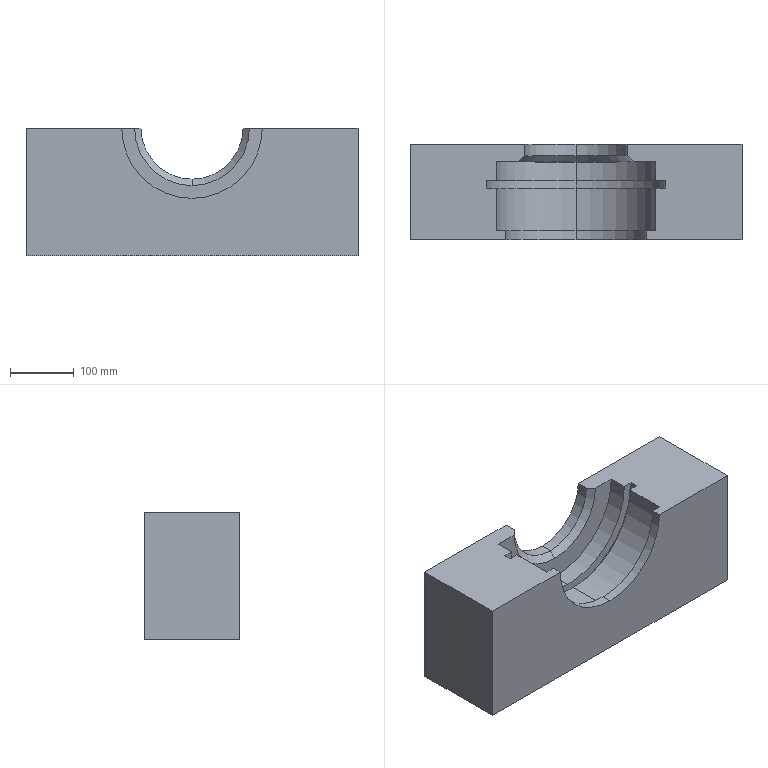Part | SolidWorks | features Chamfer 1, Extrusion 1, HoleWzd 1, RevCut 1 | 1 solid | 41 faces | box 520 x 150 x 200 mm | volume 12315251 mm3 | cylinder 16 | cone 14 | plane 11 | commonest cylinder face diameters 10.2 x6 250 x4 160 x2 220 x2 280 x2
STEP:
#1=CARTESIAN_POINT('',(-260.,132.,-80.));
#2=VERTEX_POINT('',#1);
#3=CARTESIAN_POINT('',(-180.,132.,0.));
#4=VERTEX_POINT('',#3);
#5=CARTESIAN_POINT('',(-260.,132.,0.));
#6=DIRECTION('',(0.,-1.,0.));
#7=DIRECTION('',(0.,0.,-1.));
#8=AXIS2_PLACEMENT_3D('',#5,#6,#7);
#9=CIRCLE('',#8,80.);
#10=EDGE_CURVE('',#2,#4,#9,.T.);
#11=ORIENTED_EDGE('',*,*,#10,.F.);
#12=CARTESIAN_POINT('',(-260.,122.,-90.));
#13=VERTEX_POINT('',#12);
#14=CARTESIAN_POINT('',(-260.,132.,-80.));
#15=DIRECTION('',(0.,-0.7071,-0.7071));
#16=VECTOR('',#15,1000.);
#17=LINE('',#14,#16);
#18=EDGE_CURVE('',#2,#13,#17,.T.);
#19=ORIENTED_EDGE('',*,*,#18,.T.);
#20=CARTESIAN_POINT('',(-170.,122.,0.));
#21=VERTEX_POINT('',#20);
#22=CARTESIAN_POINT('',(-260.,122.,0.));
#23=DIRECTION('',(0.,1.,0.));
#24=DIRECTION('',(0.,0.,-1.));
#25=AXIS2_PLACEMENT_3D('',#22,#23,#24);
#26=CIRCLE('',#25,90.);
#27=EDGE_CURVE('',#21,#13,#26,.T.);
#28=ORIENTED_EDGE('',*,*,#27,.F.);
#29=CARTESIAN_POINT('',(-260.,212.,0.));
#30=DIRECTION('',(0.7071,-0.7071,0.));
#31=VECTOR('',#30,1000.);
#32=LINE('',#29,#31);
#33=EDGE_CURVE('',#4,#21,#32,.T.);
#34=ORIENTED_EDGE('',*,*,#33,.F.);
#35=EDGE_LOOP('',(#11,#19,#28,#34));
#36=FACE_OUTER_BOUND('',#35,.T.);
#37=CARTESIAN_POINT('',(-260.,132.,0.));
#38=DIRECTION('',(0.,-1.,0.));
#39=DIRECTION('',(0.,0.,-1.));
#40=AXIS2_PLACEMENT_3D('',#37,#38,#39);
#41=CONICAL_SURFACE('',#40,80.,0.7854);
#42=ADVANCED_FACE('',(#36),#41,.F.);
#43=CARTESIAN_POINT('',(-260.,15.,-110.));
#44=VERTEX_POINT('',#43);
#45=CARTESIAN_POINT('',(-150.,15.,0.));
#46=VERTEX_POINT('',#45);
#47=CARTESIAN_POINT('',(-260.,15.,0.));
#48=DIRECTION('',(0.,-1.,0.));
#49=DIRECTION('',(0.,0.,-1.));
#50=AXIS2_PLACEMENT_3D('',#47,#48,#49);
#51=CIRCLE('',#50,110.);
#52=EDGE_CURVE('',#44,#46,#51,.T.);
#53=ORIENTED_EDGE('',*,*,#52,.F.);
#54=CARTESIAN_POINT('',(-260.,0.,-110.));
#55=VERTEX_POINT('',#54);
#56=CARTESIAN_POINT('',(-260.,0.,-110.));
#57=DIRECTION('',(0.,-1.,0.));
#58=VECTOR('',#57,1000.);
#59=LINE('',#56,#58);
#60=EDGE_CURVE('',#44,#55,#59,.T.);
#61=ORIENTED_EDGE('',*,*,#60,.T.);
#62=CARTESIAN_POINT('',(-150.,0.,0.));
#63=VERTEX_POINT('',#62);
#64=CARTESIAN_POINT('',(-260.,0.,0.));
#65=DIRECTION('',(0.,-1.,0.));
#66=DIRECTION('',(0.,0.,1.));
#67=AXIS2_PLACEMENT_3D('',#64,#65,#66);
#68=CIRCLE('',#67,110.);
#69=EDGE_CURVE('',#55,#63,#68,.T.);
#70=ORIENTED_EDGE('',*,*,#69,.T.);
#71=CARTESIAN_POINT('',(-150.,0.,0.));
#72=DIRECTION('',(0.,1.,0.));
#73=VECTOR('',#72,1000.);
#74=LINE('',#71,#73);
#75=EDGE_CURVE('',#63,#46,#74,.T.);
#76=ORIENTED_EDGE('',*,*,#75,.T.);
#77=EDGE_LOOP('',(#53,#61,#70,#76));
#78=FACE_OUTER_BOUND('',#77,.T.);
#79=CARTESIAN_POINT('',(-260.,0.,0.));
#80=DIRECTION('',(0.,-1.,0.));
#81=DIRECTION('',(0.,0.,-1.));
#82=AXIS2_PLACEMENT_3D('',#79,#80,#81);
#83=CYLINDRICAL_SURFACE('',#82,110.);
#84=ADVANCED_FACE('',(#78),#83,.F.);
#85=CARTESIAN_POINT('',(-260.,150.,-80.));
#86=VERTEX_POINT('',#85);
#87=CARTESIAN_POINT('',(-180.,150.,0.));
#88=VERTEX_POINT('',#87);
#89=CARTESIAN_POINT('',(-260.,150.,0.));
#90=DIRECTION('',(0.,-1.,0.));
#91=DIRECTION('',(0.,0.,1.));
#92=AXIS2_PLACEMENT_3D('',#89,#90,#91);
#93=CIRCLE('',#92,80.);
#94=EDGE_CURVE('',#86,#88,#93,.T.);
#95=ORIENTED_EDGE('',*,*,#94,.F.);
#96=CARTESIAN_POINT('',(-260.,0.,-80.));
#97=DIRECTION('',(0.,-1.,0.));
#98=VECTOR('',#97,1000.);
#99=LINE('',#96,#98);
#100=EDGE_CURVE('',#86,#2,#99,.T.);
#101=ORIENTED_EDGE('',*,*,#100,.T.);
#102=ORIENTED_EDGE('',*,*,#10,.T.);
#103=CARTESIAN_POINT('',(-180.,0.,0.));
#104=DIRECTION('',(0.,1.,0.));
#105=VECTOR('',#104,1000.);
#106=LINE('',#103,#105);
#107=EDGE_CURVE('',#4,#88,#106,.T.);
#108=ORIENTED_EDGE('',*,*,#107,.T.);
#109=EDGE_LOOP('',(#95,#101,#102,#108));
#110=FACE_OUTER_BOUND('',#109,.T.);
#111=CARTESIAN_POINT('',(-260.,0.,0.));
#112=DIRECTION('',(0.,-1.,0.));
#113=DIRECTION('',(0.,0.,-1.));
#114=AXIS2_PLACEMENT_3D('',#111,#112,#113);
#115=CYLINDRICAL_SURFACE('',#114,80.);
#116=ADVANCED_FACE('',(#110),#115,.F.);
#117=CARTESIAN_POINT('',(-260.,81.,-125.));
#118=VERTEX_POINT('',#117);
#119=CARTESIAN_POINT('',(-135.,81.,0.));
#120=VERTEX_POINT('',#119);
#121=CARTESIAN_POINT('',(-260.,81.,0.));
#122=DIRECTION('',(0.,-1.,0.));
#123=DIRECTION('',(0.,0.,-1.));
#124=AXIS2_PLACEMENT_3D('',#121,#122,#123);
#125=CIRCLE('',#124,125.);
#126=EDGE_CURVE('',#118,#120,#125,.T.);
#127=ORIENTED_EDGE('',*,*,#126,.F.);
#128=CARTESIAN_POINT('',(-260.,15.,-125.));
#129=VERTEX_POINT('',#128);
#130=CARTESIAN_POINT('',(-260.,0.,-125.));
#131=DIRECTION('',(0.,-1.,0.));
#132=VECTOR('',#131,1000.);
#133=LINE('',#130,#132);
#134=EDGE_CURVE('',#118,#129,#133,.T.);
#135=ORIENTED_EDGE('',*,*,#134,.T.);
#136=CARTESIAN_POINT('',(-135.,15.,0.));
#137=VERTEX_POINT('',#136);
#138=CARTESIAN_POINT('',(-260.,15.,0.));
#139=DIRECTION('',(0.,-1.,0.));
#140=DIRECTION('',(0.,0.,-1.));
#141=AXIS2_PLACEMENT_3D('',#138,#139,#140);
#142=CIRCLE('',#141,125.);
#143=EDGE_CURVE('',#129,#137,#142,.T.);
#144=ORIENTED_EDGE('',*,*,#143,.T.);
#145=CARTESIAN_POINT('',(-135.,0.,0.));
#146=DIRECTION('',(0.,1.,0.));
#147=VECTOR('',#146,1000.);
#148=LINE('',#145,#147);
#149=EDGE_CURVE('',#137,#120,#148,.T.);
#150=ORIENTED_EDGE('',*,*,#149,.T.);
#151=EDGE_LOOP('',(#127,#135,#144,#150));
#152=FACE_OUTER_BOUND('',#151,.T.);
#153=CARTESIAN_POINT('',(-260.,0.,0.));
#154=DIRECTION('',(0.,-1.,0.));
#155=DIRECTION('',(0.,0.,-1.));
#156=AXIS2_PLACEMENT_3D('',#153,#154,#155);
#157=CYLINDRICAL_SURFACE('',#156,125.);
#158=ADVANCED_FACE('',(#152),#157,.F.);
#159=CARTESIAN_POINT('',(-260.,93.,-140.));
#160=VERTEX_POINT('',#159);
#161=CARTESIAN_POINT('',(-120.,93.,0.));
#162=VERTEX_POINT('',#161);
#163=CARTESIAN_POINT('',(-260.,93.,0.));
#164=DIRECTION('',(0.,-1.,0.));
#165=DIRECTION('',(0.,0.,-1.));
#166=AXIS2_PLACEMENT_3D('',#163,#164,#165);
#167=CIRCLE('',#166,140.);
#168=EDGE_CURVE('',#160,#162,#167,.T.);
#169=ORIENTED_EDGE('',*,*,#168,.F.);
#170=CARTESIAN_POINT('',(-260.,81.,-140.));
#171=VERTEX_POINT('',#170);
#172=CARTESIAN_POINT('',(-260.,0.,-140.));
#173=DIRECTION('',(0.,-1.,0.));
#174=VECTOR('',#173,1000.);
#175=LINE('',#172,#174);
#176=EDGE_CURVE('',#160,#171,#175,.T.);
#177=ORIENTED_EDGE('',*,*,#176,.T.);
#178=CARTESIAN_POINT('',(-120.,81.,0.));
#179=VERTEX_POINT('',#178);
#180=CARTESIAN_POINT('',(-260.,81.,0.));
#181=DIRECTION('',(0.,-1.,0.));
#182=DIRECTION('',(0.,0.,-1.));
#183=AXIS2_PLACEMENT_3D('',#180,#181,#182);
#184=CIRCLE('',#183,140.);
#185=EDGE_CURVE('',#171,#179,#184,.T.);
#186=ORIENTED_EDGE('',*,*,#185,.T.);
#187=CARTESIAN_POINT('',(-120.,0.,0.));
#188=DIRECTION('',(0.,1.,0.));
#189=VECTOR('',#188,1000.);
#190=LINE('',#187,#189);
#191=EDGE_CURVE('',#179,#162,#190,.T.);
#192=ORIENTED_EDGE('',*,*,#191,.T.);
#193=EDGE_LOOP('',(#169,#177,#186,#192));
#194=FACE_OUTER_BOUND('',#193,.T.);
#195=CARTESIAN_POINT('',(-260.,0.,0.));
#196=DIRECTION('',(0.,-1.,0.));
#197=DIRECTION('',(0.,0.,-1.));
#198=AXIS2_PLACEMENT_3D('',#195,#196,#197);
#199=CYLINDRICAL_SURFACE('',#198,140.);
#200=ADVANCED_FACE('',(#194),#199,.F.);
#201=CARTESIAN_POINT('',(-260.,122.,-125.));
#202=VERTEX_POINT('',#201);
#203=CARTESIAN_POINT('',(-135.,122.,0.));
#204=VERTEX_POINT('',#203);
#205=CARTESIAN_POINT('',(-260.,122.,0.));
#206=DIRECTION('',(0.,-1.,0.));
#207=DIRECTION('',(0.,0.,-1.));
#208=AXIS2_PLACEMENT_3D('',#205,#206,#207);
#209=CIRCLE('',#208,125.);
#210=EDGE_CURVE('',#202,#204,#209,.T.);
#211=ORIENTED_EDGE('',*,*,#210,.F.);
#212=CARTESIAN_POINT('',(-260.,93.,-125.));
#213=VERTEX_POINT('',#212);
#214=CARTESIAN_POINT('',(-260.,0.,-125.));
#215=DIRECTION('',(0.,-1.,0.));
#216=VECTOR('',#215,1000.);
#217=LINE('',#214,#216);
#218=EDGE_CURVE('',#202,#213,#217,.T.);
#219=ORIENTED_EDGE('',*,*,#218,.T.);
#220=CARTESIAN_POINT('',(-135.,93.,0.));
#221=VERTEX_POINT('',#220);
#222=CARTESIAN_POINT('',(-260.,93.,0.));
#223=DIRECTION('',(0.,-1.,0.));
#224=DIRECTION('',(0.,0.,-1.));
#225=AXIS2_PLACEMENT_3D('',#222,#223,#224);
#226=CIRCLE('',#225,125.);
#227=EDGE_CURVE('',#213,#221,#226,.T.);
#228=ORIENTED_EDGE('',*,*,#227,.T.);
#229=CARTESIAN_POINT('',(-135.,0.,0.));
#230=DIRECTION('',(0.,1.,0.));
#231=VECTOR('',#230,1000.);
#232=LINE('',#229,#231);
#233=EDGE_CURVE('',#221,#204,#232,.T.);
#234=ORIENTED_EDGE('',*,*,#233,.T.);
#235=EDGE_LOOP('',(#211,#219,#228,#234));
#236=FACE_OUTER_BOUND('',#235,.T.);
#237=CARTESIAN_POINT('',(-260.,0.,0.));
#238=DIRECTION('',(0.,-1.,0.));
#239=DIRECTION('',(0.,0.,-1.));
#240=AXIS2_PLACEMENT_3D('',#237,#238,#239);
#241=CYLINDRICAL_SURFACE('',#240,125.);
#242=ADVANCED_FACE('',(#236),#241,.F.);
#243=CARTESIAN_POINT('',(-260.,149.075,-105.1));
#244=VERTEX_POINT('',#243);
#245=CARTESIAN_POINT('',(-260.,149.075,-94.9));
#246=VERTEX_POINT('',#245);
#247=CARTESIAN_POINT('',(-260.,149.075,-100.));
#248=DIRECTION('',(0.,1.,0.));
#249=DIRECTION('',(0.,0.,1.));
#250=AXIS2_PLACEMENT_3D('',#247,#248,#249);
#251=CIRCLE('',#250,5.1);
#252=EDGE_CURVE('',#244,#246,#251,.T.);
#253=ORIENTED_EDGE('',*,*,#252,.F.);
#254=CARTESIAN_POINT('',(-260.,150.,-106.025));
#255=VERTEX_POINT('',#254);
#256=CARTESIAN_POINT('',(-260.,150.,-106.025));
#257=DIRECTION('',(0.,0.7071,-0.7071));
#258=VECTOR('',#257,1000.);
#259=LINE('',#256,#258);
#260=EDGE_CURVE('',#244,#255,#259,.T.);
#261=ORIENTED_EDGE('',*,*,#260,.T.);
#262=CARTESIAN_POINT('',(-260.,150.,-93.975));
#263=VERTEX_POINT('',#262);
#264=CARTESIAN_POINT('',(-260.,150.,-100.));
#265=DIRECTION('',(0.,1.,0.));
#266=DIRECTION('',(0.,0.,1.));
#267=AXIS2_PLACEMENT_3D('',#264,#265,#266);
#268=CIRCLE('',#267,6.025);
#269=EDGE_CURVE('',#255,#263,#268,.T.);
#270=ORIENTED_EDGE('',*,*,#269,.T.);
#271=CARTESIAN_POINT('',(-260.,150.,-93.975));
#272=DIRECTION('',(0.,0.7071,0.7071));
#273=VECTOR('',#272,1000.);
#274=LINE('',#271,#273);
#275=EDGE_CURVE('',#246,#263,#274,.T.);
#276=ORIENTED_EDGE('',*,*,#275,.F.);
#277=EDGE_LOOP('',(#253,#261,#270,#276));
#278=FACE_OUTER_BOUND('',#277,.T.);
#279=CARTESIAN_POINT('',(-260.,150.,-100.));
#280=DIRECTION('',(0.,1.,0.));
#281=DIRECTION('',(0.,0.,1.));
#282=AXIS2_PLACEMENT_3D('',#279,#280,#281);
#283=CONICAL_SURFACE('',#282,6.025,0.7854);
#284=ADVANCED_FACE('',(#278),#283,.F.);
#285=CARTESIAN_POINT('',(-260.,135.,-105.1));
#286=VERTEX_POINT('',#285);
#287=CARTESIAN_POINT('',(-260.,135.,-94.9));
#288=VERTEX_POINT('',#287);
#289=CARTESIAN_POINT('',(-260.,135.,-100.));
#290=DIRECTION('',(0.,1.,0.));
#291=DIRECTION('',(0.,0.,1.));
#292=AXIS2_PLACEMENT_3D('',#289,#290,#291);
#293=CIRCLE('',#292,5.1);
#294=EDGE_CURVE('',#286,#288,#293,.T.);
#295=ORIENTED_EDGE('',*,*,#294,.F.);
#296=CARTESIAN_POINT('',(-260.,150.,-105.1));
#297=DIRECTION('',(0.,1.,0.));
#298=VECTOR('',#297,1000.);
#299=LINE('',#296,#298);
#300=EDGE_CURVE('',#286,#244,#299,.T.);
#301=ORIENTED_EDGE('',*,*,#300,.T.);
#302=ORIENTED_EDGE('',*,*,#252,.T.);
#303=CARTESIAN_POINT('',(-260.,150.,-94.9));
#304=DIRECTION('',(0.,1.,0.));
#305=VECTOR('',#304,1000.);
#306=LINE('',#303,#305);
#307=EDGE_CURVE('',#288,#246,#306,.T.);
#308=ORIENTED_EDGE('',*,*,#307,.F.);
#309=EDGE_LOOP('',(#295,#301,#302,#308));
#310=FACE_OUTER_BOUND('',#309,.T.);
#311=CARTESIAN_POINT('',(-260.,150.,-100.));
#312=DIRECTION('',(0.,1.,0.));
#313=DIRECTION('',(0.,0.,1.));
#314=AXIS2_PLACEMENT_3D('',#311,#312,#313);
#315=CYLINDRICAL_SURFACE('',#314,5.1);
#316=ADVANCED_FACE('',(#310),#315,.F.);
#317=CARTESIAN_POINT('',(-260.,131.936,-100.));
#318=VERTEX_POINT('',#317);
#319=CARTESIAN_POINT('',(-260.,135.,-94.9));
#320=DIRECTION('',(0.,0.515,0.8572));
#321=VECTOR('',#320,1000.);
#322=LINE('',#319,#321);
#323=EDGE_CURVE('',#318,#288,#322,.T.);
#324=ORIENTED_EDGE('',*,*,#323,.F.);
#325=CARTESIAN_POINT('',(-260.,135.,-105.1));
#326=DIRECTION('',(0.,0.515,-0.8572));
#327=VECTOR('',#326,1000.);
#328=LINE('',#325,#327);
#329=EDGE_CURVE('',#318,#286,#328,.T.);
#330=ORIENTED_EDGE('',*,*,#329,.T.);
#331=ORIENTED_EDGE('',*,*,#294,.T.);
#332=EDGE_LOOP('',(#324,#330,#331));
#333=FACE_OUTER_BOUND('',#332,.T.);
#334=CARTESIAN_POINT('',(-260.,135.,-100.));
#335=DIRECTION('',(0.,1.,0.));
#336=DIRECTION('',(0.,0.,1.));
#337=AXIS2_PLACEMENT_3D('',#334,#335,#336);
#338=CONICAL_SURFACE('',#337,5.1,1.03);
#339=ADVANCED_FACE('',(#333),#338,.F.);
#340=CARTESIAN_POINT('',(-173.397,149.075,-55.1));
#341=VERTEX_POINT('',#340);
#342=CARTESIAN_POINT('',(-173.397,149.075,-44.9));
#343=VERTEX_POINT('',#342);
#344=CARTESIAN_POINT('',(-173.397,149.075,-50.));
#345=DIRECTION('',(0.,1.,0.));
#346=DIRECTION('',(0.,0.,1.));
#347=AXIS2_PLACEMENT_3D('',#344,#345,#346);
#348=CIRCLE('',#347,5.1);
#349=EDGE_CURVE('',#341,#343,#348,.T.);
#350=ORIENTED_EDGE('',*,*,#349,.F.);
#351=CARTESIAN_POINT('',(-173.397,150.,-56.025));
#352=VERTEX_POINT('',#351);
#353=CARTESIAN_POINT('',(-173.397,150.,-56.025));
#354=DIRECTION('',(0.,0.7071,-0.7071));
#355=VECTOR('',#354,1000.);
#356=LINE('',#353,#355);
#357=EDGE_CURVE('',#341,#352,#356,.T.);
#358=ORIENTED_EDGE('',*,*,#357,.T.);
#359=CARTESIAN_POINT('',(-173.397,150.,-43.975));
#360=VERTEX_POINT('',#359);
#361=CARTESIAN_POINT('',(-173.397,150.,-50.));
#362=DIRECTION('',(0.,1.,0.));
#363=DIRECTION('',(0.,0.,1.));
#364=AXIS2_PLACEMENT_3D('',#361,#362,#363);
#365=CIRCLE('',#364,6.025);
#366=EDGE_CURVE('',#352,#360,#365,.T.);
#367=ORIENTED_EDGE('',*,*,#366,.T.);
#368=CARTESIAN_POINT('',(-173.397,150.,-43.975));
#369=DIRECTION('',(0.,0.7071,0.7071));
#370=VECTOR('',#369,1000.);
#371=LINE('',#368,#370);
#372=EDGE_CURVE('',#343,#360,#371,.T.);
#373=ORIENTED_EDGE('',*,*,#372,.F.);
#374=EDGE_LOOP('',(#350,#358,#367,#373));
#375=FACE_OUTER_BOUND('',#374,.T.);
#376=CARTESIAN_POINT('',(-173.397,150.,-50.));
#377=DIRECTION('',(0.,1.,0.));
#378=DIRECTION('',(0.,0.,1.));
#379=AXIS2_PLACEMENT_3D('',#376,#377,#378);
#380=CONICAL_SURFACE('',#379,6.025,0.7854);
#381=ADVANCED_FACE('',(#375),#380,.F.);
#382=CARTESIAN_POINT('',(-173.397,135.,-55.1));
#383=VERTEX_POINT('',#382);
#384=CARTESIAN_POINT('',(-173.397,135.,-44.9));
#385=VERTEX_POINT('',#384);
#386=CARTESIAN_POINT('',(-173.397,135.,-50.));
#387=DIRECTION('',(0.,1.,0.));
#388=DIRECTION('',(0.,0.,1.));
#389=AXIS2_PLACEMENT_3D('',#386,#387,#388);
#390=CIRCLE('',#389,5.1);
#391=EDGE_CURVE('',#383,#385,#390,.T.);
#392=ORIENTED_EDGE('',*,*,#391,.F.);
#393=CARTESIAN_POINT('',(-173.397,150.,-55.1));
#394=DIRECTION('',(0.,1.,0.));
#395=VECTOR('',#394,1000.);
#396=LINE('',#393,#395);
#397=EDGE_CURVE('',#383,#341,#396,.T.);
#398=ORIENTED_EDGE('',*,*,#397,.T.);
#399=ORIENTED_EDGE('',*,*,#349,.T.);
#400=CARTESIAN_POINT('',(-173.397,150.,-44.9));
#401=DIRECTION('',(0.,1.,0.));
#402=VECTOR('',#401,1000.);
#403=LINE('',#400,#402);
#404=EDGE_CURVE('',#385,#343,#403,.T.);
#405=ORIENTED_EDGE('',*,*,#404,.F.);
#406=EDGE_LOOP('',(#392,#398,#399,#405));
#407=FACE_OUTER_BOUND('',#406,.T.);
#408=CARTESIAN_POINT('',(-173.397,150.,-50.));
#409=DIRECTION('',(0.,1.,0.));
#410=DIRECTION('',(0.,0.,1.));
#411=AXIS2_PLACEMENT_3D('',#408,#409,#410);
#412=CYLINDRICAL_SURFACE('',#411,5.1);
#413=ADVANCED_FACE('',(#407),#412,.F.);
#414=CARTESIAN_POINT('',(-173.397,131.936,-50.));
#415=VERTEX_POINT('',#414);
#416=CARTESIAN_POINT('',(-173.397,135.,-44.9));
#417=DIRECTION('',(0.,0.515,0.8572));
#418=VECTOR('',#417,1000.);
#419=LINE('',#416,#418);
#420=EDGE_CURVE('',#415,#385,#419,.T.);
#421=ORIENTED_EDGE('',*,*,#420,.F.);
#422=CARTESIAN_POINT('',(-173.397,135.,-55.1));
#423=DIRECTION('',(0.,0.515,-0.8572));
#424=VECTOR('',#423,1000.);
#425=LINE('',#422,#424);
#426=EDGE_CURVE('',#415,#383,#425,.T.);
#427=ORIENTED_EDGE('',*,*,#426,.T.);
#428=ORIENTED_EDGE('',*,*,#391,.T.);
#429=EDGE_LOOP('',(#421,#427,#428));
#430=FACE_OUTER_BOUND('',#429,.T.);
#431=CARTESIAN_POINT('',(-173.397,135.,-50.));
#432=DIRECTION('',(0.,1.,0.));
#433=DIRECTION('',(0.,0.,1.));
#434=AXIS2_PLACEMENT_3D('',#431,#432,#433);
#435=CONICAL_SURFACE('',#434,5.1,1.03);
#436=ADVANCED_FACE('',(#430),#435,.F.);
#437=CARTESIAN_POINT('',(-346.603,149.075,-55.1));
#438=VERTEX_POINT('',#437);
#439=CARTESIAN_POINT('',(-346.603,149.075,-44.9));
#440=VERTEX_POINT('',#439);
#441=CARTESIAN_POINT('',(-346.603,149.075,-50.));
#442=DIRECTION('',(0.,1.,0.));
#443=DIRECTION('',(0.,0.,1.));
#444=AXIS2_PLACEMENT_3D('',#441,#442,#443);
#445=CIRCLE('',#444,5.1);
#446=EDGE_CURVE('',#438,#440,#445,.T.);
#447=ORIENTED_EDGE('',*,*,#446,.F.);
#448=CARTESIAN_POINT('',(-346.603,150.,-56.025));
#449=VERTEX_POINT('',#448);
#450=CARTESIAN_POINT('',(-346.603,150.,-56.025));
#451=DIRECTION('',(0.,0.7071,-0.7071));
#452=VECTOR('',#451,1000.);
#453=LINE('',#450,#452);
#454=EDGE_CURVE('',#438,#449,#453,.T.);
#455=ORIENTED_EDGE('',*,*,#454,.T.);
#456=CARTESIAN_POINT('',(-346.603,150.,-43.975));
#457=VERTEX_POINT('',#456);
#458=CARTESIAN_POINT('',(-346.603,150.,-50.));
#459=DIRECTION('',(0.,1.,0.));
#460=DIRECTION('',(0.,0.,1.));
#461=AXIS2_PLACEMENT_3D('',#458,#459,#460);
#462=CIRCLE('',#461,6.025);
#463=EDGE_CURVE('',#449,#457,#462,.T.);
#464=ORIENTED_EDGE('',*,*,#463,.T.);
#465=CARTESIAN_POINT('',(-346.603,150.,-43.975));
#466=DIRECTION('',(0.,0.7071,0.7071));
#467=VECTOR('',#466,1000.);
#468=LINE('',#465,#467);
#469=EDGE_CURVE('',#440,#457,#468,.T.);
#470=ORIENTED_EDGE('',*,*,#469,.F.);
#471=EDGE_LOOP('',(#447,#455,#464,#470));
#472=FACE_OUTER_BOUND('',#471,.T.);
#473=CARTESIAN_POINT('',(-346.603,150.,-50.));
#474=DIRECTION('',(0.,1.,0.));
#475=DIRECTION('',(0.,0.,1.));
#476=AXIS2_PLACEMENT_3D('',#473,#474,#475);
#477=CONICAL_SURFACE('',#476,6.025,0.7854);
#478=ADVANCED_FACE('',(#472),#477,.F.);
#479=CARTESIAN_POINT('',(-346.603,135.,-55.1));
#480=VERTEX_POINT('',#479);
#481=CARTESIAN_POINT('',(-346.603,135.,-44.9));
#482=VERTEX_POINT('',#481);
#483=CARTESIAN_POINT('',(-346.603,135.,-50.));
#484=DIRECTION('',(0.,1.,0.));
#485=DIRECTION('',(0.,0.,1.));
#486=AXIS2_PLACEMENT_3D('',#483,#484,#485);
#487=CIRCLE('',#486,5.1);
#488=EDGE_CURVE('',#480,#482,#487,.T.);
#489=ORIENTED_EDGE('',*,*,#488,.F.);
#490=CARTESIAN_POINT('',(-346.603,150.,-55.1));
#491=DIRECTION('',(0.,1.,0.));
#492=VECTOR('',#491,1000.);
#493=LINE('',#490,#492);
#494=EDGE_CURVE('',#480,#438,#493,.T.);
#495=ORIENTED_EDGE('',*,*,#494,.T.);
#496=ORIENTED_EDGE('',*,*,#446,.T.);
#497=CARTESIAN_POINT('',(-346.603,150.,-44.9));
#498=DIRECTION('',(0.,1.,0.));
#499=VECTOR('',#498,1000.);
#500=LINE('',#497,#499);
#501=EDGE_CURVE('',#482,#440,#500,.T.);
#502=ORIENTED_EDGE('',*,*,#501,.F.);
#503=EDGE_LOOP('',(#489,#495,#496,#502));
#504=FACE_OUTER_BOUND('',#503,.T.);
#505=CARTESIAN_POINT('',(-346.603,150.,-50.));
#506=DIRECTION('',(0.,1.,0.));
#507=DIRECTION('',(0.,0.,1.));
#508=AXIS2_PLACEMENT_3D('',#505,#506,#507);
#509=CYLINDRICAL_SURFACE('',#508,5.1);
#510=ADVANCED_FACE('',(#504),#509,.F.);
#511=CARTESIAN_POINT('',(-346.603,131.936,-50.));
#512=VERTEX_POINT('',#511);
#513=CARTESIAN_POINT('',(-346.603,135.,-44.9));
#514=DIRECTION('',(0.,0.515,0.8572));
#515=VECTOR('',#514,1000.);
#516=LINE('',#513,#515);
#517=EDGE_CURVE('',#512,#482,#516,.T.);
#518=ORIENTED_EDGE('',*,*,#517,.F.);
#519=CARTESIAN_POINT('',(-346.603,135.,-55.1));
#520=DIRECTION('',(0.,0.515,-0.8572));
#521=VECTOR('',#520,1000.);
#522=LINE('',#519,#521);
#523=EDGE_CURVE('',#512,#480,#522,.T.);
#524=ORIENTED_EDGE('',*,*,#523,.T.);
#525=ORIENTED_EDGE('',*,*,#488,.T.);
#526=EDGE_LOOP('',(#518,#524,#525));
#527=FACE_OUTER_BOUND('',#526,.T.);
#528=CARTESIAN_POINT('',(-346.603,135.,-50.));
#529=DIRECTION('',(0.,1.,0.));
#530=DIRECTION('',(0.,0.,1.));
#531=AXIS2_PLACEMENT_3D('',#528,#529,#530);
#532=CONICAL_SURFACE('',#531,5.1,1.03);
#533=ADVANCED_FACE('',(#527),#532,.F.);
#534=ORIENTED_EDGE('',*,*,#107,.F.);
#535=ORIENTED_EDGE('',*,*,#33,.T.);
#536=CARTESIAN_POINT('',(0.,122.,0.));
#537=DIRECTION('',(-1.,0.,0.));
#538=VECTOR('',#537,1000.);
#539=LINE('',#536,#538);
#540=EDGE_CURVE('',#204,#21,#539,.T.);
#541=ORIENTED_EDGE('',*,*,#540,.F.);
#542=ORIENTED_EDGE('',*,*,#233,.F.);
#543=CARTESIAN_POINT('',(0.,93.,0.));
#544=DIRECTION('',(-1.,0.,0.));
#545=VECTOR('',#544,1000.);
#546=LINE('',#543,#545);
#547=EDGE_CURVE('',#162,#221,#546,.T.);
#548=ORIENTED_EDGE('',*,*,#547,.F.);
#549=ORIENTED_EDGE('',*,*,#191,.F.);
#550=CARTESIAN_POINT('',(0.,81.,0.));
#551=DIRECTION('',(1.,0.,0.));
#552=VECTOR('',#551,1000.);
#553=LINE('',#550,#552);
#554=EDGE_CURVE('',#120,#179,#553,.T.);
#555=ORIENTED_EDGE('',*,*,#554,.F.);
#556=ORIENTED_EDGE('',*,*,#149,.F.);
#557=CARTESIAN_POINT('',(0.,15.,0.));
#558=DIRECTION('',(1.,0.,0.));
#559=VECTOR('',#558,1000.);
#560=LINE('',#557,#559);
#561=EDGE_CURVE('',#46,#137,#560,.T.);
#562=ORIENTED_EDGE('',*,*,#561,.F.);
#563=ORIENTED_EDGE('',*,*,#75,.F.);
#564=CARTESIAN_POINT('',(0.,0.,0.));
#565=VERTEX_POINT('',#564);
#566=CARTESIAN_POINT('',(0.,0.,0.));
#567=DIRECTION('',(1.,0.,0.));
#568=VECTOR('',#567,1000.);
#569=LINE('',#566,#568);
#570=EDGE_CURVE('',#63,#565,#569,.T.);
#571=ORIENTED_EDGE('',*,*,#570,.T.);
#572=CARTESIAN_POINT('',(0.,150.,0.));
#573=VERTEX_POINT('',#572);
#574=CARTESIAN_POINT('',(0.,150.,0.));
#575=DIRECTION('',(0.,-1.,0.));
#576=VECTOR('',#575,1000.);
#577=LINE('',#574,#576);
#578=EDGE_CURVE('',#573,#565,#577,.T.);
#579=ORIENTED_EDGE('',*,*,#578,.F.);
#580=CARTESIAN_POINT('',(0.,150.,0.));
#581=DIRECTION('',(1.,0.,0.));
#582=VECTOR('',#581,1000.);
#583=LINE('',#580,#582);
#584=EDGE_CURVE('',#88,#573,#583,.T.);
#585=ORIENTED_EDGE('',*,*,#584,.F.);
#586=EDGE_LOOP('',(#534,#535,#541,#542,#548,#549,#555,#556,#562,#563,#571,#579,#585));
#587=FACE_OUTER_BOUND('',#586,.T.);
#588=CARTESIAN_POINT('',(0.,150.,0.));
#589=DIRECTION('',(0.,0.,-1.));
#590=DIRECTION('',(-1.,0.,0.));
#591=AXIS2_PLACEMENT_3D('',#588,#589,#590);
#592=PLANE('',#591);
#593=ADVANCED_FACE('',(#587),#592,.F.);
#594=CARTESIAN_POINT('',(-350.,122.,0.));
#595=VERTEX_POINT('',#594);
#596=CARTESIAN_POINT('',(-385.,122.,0.));
#597=VERTEX_POINT('',#596);
#598=CARTESIAN_POINT('',(0.,122.,0.));
#599=DIRECTION('',(-1.,0.,0.));
#600=VECTOR('',#599,1000.);
#601=LINE('',#598,#600);
#602=EDGE_CURVE('',#595,#597,#601,.T.);
#603=ORIENTED_EDGE('',*,*,#602,.F.);
#604=CARTESIAN_POINT('',(-340.,132.,0.));
#605=VERTEX_POINT('',#604);
#606=CARTESIAN_POINT('',(-260.,212.,0.));
#607=DIRECTION('',(0.7071,0.7071,0.));
#608=VECTOR('',#607,1000.);
#609=LINE('',#606,#608);
#610=EDGE_CURVE('',#595,#605,#609,.T.);
#611=ORIENTED_EDGE('',*,*,#610,.T.);
#612=CARTESIAN_POINT('',(-340.,150.,0.));
#613=VERTEX_POINT('',#612);
#614=CARTESIAN_POINT('',(-340.,0.,0.));
#615=DIRECTION('',(0.,-1.,0.));
#616=VECTOR('',#615,1000.);
#617=LINE('',#614,#616);
#618=EDGE_CURVE('',#613,#605,#617,.T.);
#619=ORIENTED_EDGE('',*,*,#618,.F.);
#620=CARTESIAN_POINT('',(-520.,150.,0.));
#621=VERTEX_POINT('',#620);
#622=CARTESIAN_POINT('',(0.,150.,0.));
#623=DIRECTION('',(1.,0.,0.));
#624=VECTOR('',#623,1000.);
#625=LINE('',#622,#624);
#626=EDGE_CURVE('',#621,#613,#625,.T.);
#627=ORIENTED_EDGE('',*,*,#626,.F.);
#628=CARTESIAN_POINT('',(-520.,0.,0.));
#629=VERTEX_POINT('',#628);
#630=CARTESIAN_POINT('',(-520.,150.,0.));
#631=DIRECTION('',(0.,-1.,0.));
#632=VECTOR('',#631,1000.);
#633=LINE('',#630,#632);
#634=EDGE_CURVE('',#621,#629,#633,.T.);
#635=ORIENTED_EDGE('',*,*,#634,.T.);
#636=CARTESIAN_POINT('',(-370.,0.,0.));
#637=VERTEX_POINT('',#636);
#638=CARTESIAN_POINT('',(0.,0.,0.));
#639=DIRECTION('',(1.,0.,0.));
#640=VECTOR('',#639,1000.);
#641=LINE('',#638,#640);
#642=EDGE_CURVE('',#629,#637,#641,.T.);
#643=ORIENTED_EDGE('',*,*,#642,.T.);
#644=CARTESIAN_POINT('',(-370.,15.,0.));
#645=VERTEX_POINT('',#644);
#646=CARTESIAN_POINT('',(-370.,0.,0.));
#647=DIRECTION('',(0.,-1.,0.));
#648=VECTOR('',#647,1000.);
#649=LINE('',#646,#648);
#650=EDGE_CURVE('',#645,#637,#649,.T.);
#651=ORIENTED_EDGE('',*,*,#650,.F.);
#652=CARTESIAN_POINT('',(-385.,15.,0.));
#653=VERTEX_POINT('',#652);
#654=CARTESIAN_POINT('',(0.,15.,0.));
#655=DIRECTION('',(1.,0.,0.));
#656=VECTOR('',#655,1000.);
#657=LINE('',#654,#656);
#658=EDGE_CURVE('',#653,#645,#657,.T.);
#659=ORIENTED_EDGE('',*,*,#658,.F.);
#660=CARTESIAN_POINT('',(-385.,81.,0.));
#661=VERTEX_POINT('',#660);
#662=CARTESIAN_POINT('',(-385.,0.,0.));
#663=DIRECTION('',(0.,-1.,0.));
#664=VECTOR('',#663,1000.);
#665=LINE('',#662,#664);
#666=EDGE_CURVE('',#661,#653,#665,.T.);
#667=ORIENTED_EDGE('',*,*,#666,.F.);
#668=CARTESIAN_POINT('',(-400.,81.,0.));
#669=VERTEX_POINT('',#668);
#670=CARTESIAN_POINT('',(0.,81.,0.));
#671=DIRECTION('',(1.,0.,0.));
#672=VECTOR('',#671,1000.);
#673=LINE('',#670,#672);
#674=EDGE_CURVE('',#669,#661,#673,.T.);
#675=ORIENTED_EDGE('',*,*,#674,.F.);
#676=CARTESIAN_POINT('',(-400.,93.,0.));
#677=VERTEX_POINT('',#676);
#678=CARTESIAN_POINT('',(-400.,0.,0.));
#679=DIRECTION('',(0.,-1.,0.));
#680=VECTOR('',#679,1000.);
#681=LINE('',#678,#680);
#682=EDGE_CURVE('',#677,#669,#681,.T.);
#683=ORIENTED_EDGE('',*,*,#682,.F.);
#684=CARTESIAN_POINT('',(-385.,93.,0.));
#685=VERTEX_POINT('',#684);
#686=CARTESIAN_POINT('',(0.,93.,0.));
#687=DIRECTION('',(-1.,0.,0.));
#688=VECTOR('',#687,1000.);
#689=LINE('',#686,#688);
#690=EDGE_CURVE('',#685,#677,#689,.T.);
#691=ORIENTED_EDGE('',*,*,#690,.F.);
#692=CARTESIAN_POINT('',(-385.,0.,0.));
#693=DIRECTION('',(0.,-1.,0.));
#694=VECTOR('',#693,1000.);
#695=LINE('',#692,#694);
#696=EDGE_CURVE('',#597,#685,#695,.T.);
#697=ORIENTED_EDGE('',*,*,#696,.F.);
#698=EDGE_LOOP('',(#603,#611,#619,#627,#635,#643,#651,#659,#667,#675,#683,#691,#697));
#699=FACE_OUTER_BOUND('',#698,.T.);
#700=CARTESIAN_POINT('',(0.,150.,0.));
#701=DIRECTION('',(0.,0.,-1.));
#702=DIRECTION('',(-1.,0.,0.));
#703=AXIS2_PLACEMENT_3D('',#700,#701,#702);
#704=PLANE('',#703);
#705=ADVANCED_FACE('',(#699),#704,.F.);
#706=CARTESIAN_POINT('',(0.,0.,-200.));
#707=VERTEX_POINT('',#706);
#708=CARTESIAN_POINT('',(0.,0.,0.));
#709=DIRECTION('',(0.,0.,-1.));
#710=VECTOR('',#709,1000.);
#711=LINE('',#708,#710);
#712=EDGE_CURVE('',#565,#707,#711,.T.);
#713=ORIENTED_EDGE('',*,*,#712,.T.);
#714=CARTESIAN_POINT('',(0.,150.,-200.));
#715=VERTEX_POINT('',#714);
#716=CARTESIAN_POINT('',(0.,150.,-200.));
#717=DIRECTION('',(0.,-1.,0.));
#718=VECTOR('',#717,1000.);
#719=LINE('',#716,#718);
#720=EDGE_CURVE('',#715,#707,#719,.T.);
#721=ORIENTED_EDGE('',*,*,#720,.F.);
#722=CARTESIAN_POINT('',(0.,150.,0.));
#723=DIRECTION('',(0.,0.,-1.));
#724=VECTOR('',#723,1000.);
#725=LINE('',#722,#724);
#726=EDGE_CURVE('',#573,#715,#725,.T.);
#727=ORIENTED_EDGE('',*,*,#726,.F.);
#728=ORIENTED_EDGE('',*,*,#578,.T.);
#729=EDGE_LOOP('',(#713,#721,#727,#728));
#730=FACE_OUTER_BOUND('',#729,.T.);
#731=CARTESIAN_POINT('',(0.,150.,0.));
#732=DIRECTION('',(-1.,0.,0.));
#733=DIRECTION('',(0.,0.,1.));
#734=AXIS2_PLACEMENT_3D('',#731,#732,#733);
#735=PLANE('',#734);
#736=ADVANCED_FACE('',(#730),#735,.F.);
#737=CARTESIAN_POINT('',(-520.,0.,-200.));
#738=VERTEX_POINT('',#737);
#739=CARTESIAN_POINT('',(0.,0.,-200.));
#740=DIRECTION('',(-1.,0.,0.));
#741=VECTOR('',#740,1000.);
#742=LINE('',#739,#741);
#743=EDGE_CURVE('',#707,#738,#742,.T.);
#744=ORIENTED_EDGE('',*,*,#743,.T.);
#745=CARTESIAN_POINT('',(-520.,150.,-200.));
#746=VERTEX_POINT('',#745);
#747=CARTESIAN_POINT('',(-520.,150.,-200.));
#748=DIRECTION('',(0.,-1.,0.));
#749=VECTOR('',#748,1000.);
#750=LINE('',#747,#749);
#751=EDGE_CURVE('',#746,#738,#750,.T.);
#752=ORIENTED_EDGE('',*,*,#751,.F.);
#753=CARTESIAN_POINT('',(0.,150.,-200.));
#754=DIRECTION('',(-1.,0.,0.));
#755=VECTOR('',#754,1000.);
#756=LINE('',#753,#755);
#757=EDGE_CURVE('',#715,#746,#756,.T.);
#758=ORIENTED_EDGE('',*,*,#757,.F.);
#759=ORIENTED_EDGE('',*,*,#720,.T.);
#760=EDGE_LOOP('',(#744,#752,#758,#759));
#761=FACE_OUTER_BOUND('',#760,.T.);
#762=CARTESIAN_POINT('',(0.,150.,-200.));
#763=DIRECTION('',(0.,0.,1.));
#764=DIRECTION('',(1.,0.,0.));
#765=AXIS2_PLACEMENT_3D('',#762,#763,#764);
#766=PLANE('',#765);
#767=ADVANCED_FACE('',(#761),#766,.F.);
#768=CARTESIAN_POINT('',(-520.,0.,0.));
#769=DIRECTION('',(0.,0.,1.));
#770=VECTOR('',#769,1000.);
#771=LINE('',#768,#770);
#772=EDGE_CURVE('',#738,#629,#771,.T.);
#773=ORIENTED_EDGE('',*,*,#772,.T.);
#774=ORIENTED_EDGE('',*,*,#634,.F.);
#775=CARTESIAN_POINT('',(-520.,150.,0.));
#776=DIRECTION('',(0.,0.,1.));
#777=VECTOR('',#776,1000.);
#778=LINE('',#775,#777);
#779=EDGE_CURVE('',#746,#621,#778,.T.);
#780=ORIENTED_EDGE('',*,*,#779,.F.);
#781=ORIENTED_EDGE('',*,*,#751,.T.);
#782=EDGE_LOOP('',(#773,#774,#780,#781));
#783=FACE_OUTER_BOUND('',#782,.T.);
#784=CARTESIAN_POINT('',(-520.,150.,0.));
#785=DIRECTION('',(1.,0.,0.));
#786=DIRECTION('',(0.,0.,-1.));
#787=AXIS2_PLACEMENT_3D('',#784,#785,#786);
#788=PLANE('',#787);
#789=ADVANCED_FACE('',(#783),#788,.F.);
#790=CARTESIAN_POINT('',(-260.,150.,-100.));
#791=DIRECTION('',(0.,1.,0.));
#792=DIRECTION('',(0.,0.,1.));
#793=AXIS2_PLACEMENT_3D('',#790,#791,#792);
#794=CIRCLE('',#793,6.025);
#795=EDGE_CURVE('',#263,#255,#794,.T.);
#796=ORIENTED_EDGE('',*,*,#795,.F.);
#797=ORIENTED_EDGE('',*,*,#269,.F.);
#798=EDGE_LOOP('',(#796,#797));
#799=FACE_BOUND('',#798,.T.);
#800=CARTESIAN_POINT('',(-173.397,150.,-50.));
#801=DIRECTION('',(0.,1.,0.));
#802=DIRECTION('',(0.,0.,1.));
#803=AXIS2_PLACEMENT_3D('',#800,#801,#802);
#804=CIRCLE('',#803,6.025);
#805=EDGE_CURVE('',#360,#352,#804,.T.);
#806=ORIENTED_EDGE('',*,*,#805,.F.);
#807=ORIENTED_EDGE('',*,*,#366,.F.);
#808=EDGE_LOOP('',(#806,#807));
#809=FACE_BOUND('',#808,.T.);
#810=CARTESIAN_POINT('',(-346.603,150.,-50.));
#811=DIRECTION('',(0.,1.,0.));
#812=DIRECTION('',(0.,0.,1.));
#813=AXIS2_PLACEMENT_3D('',#810,#811,#812);
#814=CIRCLE('',#813,6.025);
#815=EDGE_CURVE('',#457,#449,#814,.T.);
#816=ORIENTED_EDGE('',*,*,#815,.F.);
#817=ORIENTED_EDGE('',*,*,#463,.F.);
#818=EDGE_LOOP('',(#816,#817));
#819=FACE_BOUND('',#818,.T.);
#820=ORIENTED_EDGE('',*,*,#626,.T.);
#821=CARTESIAN_POINT('',(-260.,150.,0.));
#822=DIRECTION('',(0.,-1.,0.));
#823=DIRECTION('',(0.,0.,1.));
#824=AXIS2_PLACEMENT_3D('',#821,#822,#823);
#825=CIRCLE('',#824,80.);
#826=EDGE_CURVE('',#613,#86,#825,.T.);
#827=ORIENTED_EDGE('',*,*,#826,.T.);
#828=ORIENTED_EDGE('',*,*,#94,.T.);
#829=ORIENTED_EDGE('',*,*,#584,.T.);
#830=ORIENTED_EDGE('',*,*,#726,.T.);
#831=ORIENTED_EDGE('',*,*,#757,.T.);
#832=ORIENTED_EDGE('',*,*,#779,.T.);
#833=EDGE_LOOP('',(#820,#827,#828,#829,#830,#831,#832));
#834=FACE_OUTER_BOUND('',#833,.T.);
#835=CARTESIAN_POINT('',(0.,150.,0.));
#836=DIRECTION('',(0.,1.,0.));
#837=DIRECTION('',(0.,0.,1.));
#838=AXIS2_PLACEMENT_3D('',#835,#836,#837);
#839=PLANE('',#838);
#840=ADVANCED_FACE('',(#799,#809,#819,#834),#839,.T.);
#841=CARTESIAN_POINT('',(-260.,0.,0.));
#842=DIRECTION('',(0.,-1.,0.));
#843=DIRECTION('',(0.,0.,1.));
#844=AXIS2_PLACEMENT_3D('',#841,#842,#843);
#845=CIRCLE('',#844,110.);
#846=EDGE_CURVE('',#637,#55,#845,.T.);
#847=ORIENTED_EDGE('',*,*,#846,.F.);
#848=ORIENTED_EDGE('',*,*,#642,.F.);
#849=ORIENTED_EDGE('',*,*,#772,.F.);
#850=ORIENTED_EDGE('',*,*,#743,.F.);
#851=ORIENTED_EDGE('',*,*,#712,.F.);
#852=ORIENTED_EDGE('',*,*,#570,.F.);
#853=ORIENTED_EDGE('',*,*,#69,.F.);
#854=EDGE_LOOP('',(#847,#848,#849,#850,#851,#852,#853));
#855=FACE_OUTER_BOUND('',#854,.T.);
#856=CARTESIAN_POINT('',(0.,0.,0.));
#857=DIRECTION('',(0.,1.,0.));
#858=DIRECTION('',(0.,0.,1.));
#859=AXIS2_PLACEMENT_3D('',#856,#857,#858);
#860=PLANE('',#859);
#861=ADVANCED_FACE('',(#855),#860,.F.);
#862=ORIENTED_EDGE('',*,*,#523,.F.);
#863=ORIENTED_EDGE('',*,*,#517,.T.);
#864=CARTESIAN_POINT('',(-346.603,135.,-50.));
#865=DIRECTION('',(0.,1.,0.));
#866=DIRECTION('',(0.,0.,1.));
#867=AXIS2_PLACEMENT_3D('',#864,#865,#866);
#868=CIRCLE('',#867,5.1);
#869=EDGE_CURVE('',#482,#480,#868,.T.);
#870=ORIENTED_EDGE('',*,*,#869,.T.);
#871=EDGE_LOOP('',(#862,#863,#870));
#872=FACE_OUTER_BOUND('',#871,.T.);
#873=CARTESIAN_POINT('',(-346.603,135.,-50.));
#874=DIRECTION('',(0.,1.,0.));
#875=DIRECTION('',(0.,0.,1.));
#876=AXIS2_PLACEMENT_3D('',#873,#874,#875);
#877=CONICAL_SURFACE('',#876,5.1,1.03);
#878=ADVANCED_FACE('',(#872),#877,.F.);
#879=ORIENTED_EDGE('',*,*,#494,.F.);
#880=ORIENTED_EDGE('',*,*,#869,.F.);
#881=ORIENTED_EDGE('',*,*,#501,.T.);
#882=CARTESIAN_POINT('',(-346.603,149.075,-50.));
#883=DIRECTION('',(0.,1.,0.));
#884=DIRECTION('',(0.,0.,1.));
#885=AXIS2_PLACEMENT_3D('',#882,#883,#884);
#886=CIRCLE('',#885,5.1);
#887=EDGE_CURVE('',#440,#438,#886,.T.);
#888=ORIENTED_EDGE('',*,*,#887,.T.);
#889=EDGE_LOOP('',(#879,#880,#881,#888));
#890=FACE_OUTER_BOUND('',#889,.T.);
#891=CARTESIAN_POINT('',(-346.603,150.,-50.));
#892=DIRECTION('',(0.,1.,0.));
#893=DIRECTION('',(0.,0.,1.));
#894=AXIS2_PLACEMENT_3D('',#891,#892,#893);
#895=CYLINDRICAL_SURFACE('',#894,5.1);
#896=ADVANCED_FACE('',(#890),#895,.F.);
#897=ORIENTED_EDGE('',*,*,#454,.F.);
#898=ORIENTED_EDGE('',*,*,#887,.F.);
#899=ORIENTED_EDGE('',*,*,#469,.T.);
#900=ORIENTED_EDGE('',*,*,#815,.T.);
#901=EDGE_LOOP('',(#897,#898,#899,#900));
#902=FACE_OUTER_BOUND('',#901,.T.);
#903=CARTESIAN_POINT('',(-346.603,150.,-50.));
#904=DIRECTION('',(0.,1.,0.));
#905=DIRECTION('',(0.,0.,1.));
#906=AXIS2_PLACEMENT_3D('',#903,#904,#905);
#907=CONICAL_SURFACE('',#906,6.025,0.7854);
#908=ADVANCED_FACE('',(#902),#907,.F.);
#909=ORIENTED_EDGE('',*,*,#426,.F.);
#910=ORIENTED_EDGE('',*,*,#420,.T.);
#911=CARTESIAN_POINT('',(-173.397,135.,-50.));
#912=DIRECTION('',(0.,1.,0.));
#913=DIRECTION('',(0.,0.,1.));
#914=AXIS2_PLACEMENT_3D('',#911,#912,#913);
#915=CIRCLE('',#914,5.1);
#916=EDGE_CURVE('',#385,#383,#915,.T.);
#917=ORIENTED_EDGE('',*,*,#916,.T.);
#918=EDGE_LOOP('',(#909,#910,#917));
#919=FACE_OUTER_BOUND('',#918,.T.);
#920=CARTESIAN_POINT('',(-173.397,135.,-50.));
#921=DIRECTION('',(0.,1.,0.));
#922=DIRECTION('',(0.,0.,1.));
#923=AXIS2_PLACEMENT_3D('',#920,#921,#922);
#924=CONICAL_SURFACE('',#923,5.1,1.03);
#925=ADVANCED_FACE('',(#919),#924,.F.);
#926=ORIENTED_EDGE('',*,*,#397,.F.);
#927=ORIENTED_EDGE('',*,*,#916,.F.);
#928=ORIENTED_EDGE('',*,*,#404,.T.);
#929=CARTESIAN_POINT('',(-173.397,149.075,-50.));
#930=DIRECTION('',(0.,1.,0.));
#931=DIRECTION('',(0.,0.,1.));
#932=AXIS2_PLACEMENT_3D('',#929,#930,#931);
#933=CIRCLE('',#932,5.1);
#934=EDGE_CURVE('',#343,#341,#933,.T.);
#935=ORIENTED_EDGE('',*,*,#934,.T.);
#936=EDGE_LOOP('',(#926,#927,#928,#935));
#937=FACE_OUTER_BOUND('',#936,.T.);
#938=CARTESIAN_POINT('',(-173.397,150.,-50.));
#939=DIRECTION('',(0.,1.,0.));
#940=DIRECTION('',(0.,0.,1.));
#941=AXIS2_PLACEMENT_3D('',#938,#939,#940);
#942=CYLINDRICAL_SURFACE('',#941,5.1);
#943=ADVANCED_FACE('',(#937),#942,.F.);
#944=ORIENTED_EDGE('',*,*,#357,.F.);
#945=ORIENTED_EDGE('',*,*,#934,.F.);
#946=ORIENTED_EDGE('',*,*,#372,.T.);
#947=ORIENTED_EDGE('',*,*,#805,.T.);
#948=EDGE_LOOP('',(#944,#945,#946,#947));
#949=FACE_OUTER_BOUND('',#948,.T.);
#950=CARTESIAN_POINT('',(-173.397,150.,-50.));
#951=DIRECTION('',(0.,1.,0.));
#952=DIRECTION('',(0.,0.,1.));
#953=AXIS2_PLACEMENT_3D('',#950,#951,#952);
#954=CONICAL_SURFACE('',#953,6.025,0.7854);
#955=ADVANCED_FACE('',(#949),#954,.F.);
#956=ORIENTED_EDGE('',*,*,#329,.F.);
#957=ORIENTED_EDGE('',*,*,#323,.T.);
#958=CARTESIAN_POINT('',(-260.,135.,-100.));
#959=DIRECTION('',(0.,1.,0.));
#960=DIRECTION('',(0.,0.,1.));
#961=AXIS2_PLACEMENT_3D('',#958,#959,#960);
#962=CIRCLE('',#961,5.1);
#963=EDGE_CURVE('',#288,#286,#962,.T.);
#964=ORIENTED_EDGE('',*,*,#963,.T.);
#965=EDGE_LOOP('',(#956,#957,#964));
#966=FACE_OUTER_BOUND('',#965,.T.);
#967=CARTESIAN_POINT('',(-260.,135.,-100.));
#968=DIRECTION('',(0.,1.,0.));
#969=DIRECTION('',(0.,0.,1.));
#970=AXIS2_PLACEMENT_3D('',#967,#968,#969);
#971=CONICAL_SURFACE('',#970,5.1,1.03);
#972=ADVANCED_FACE('',(#966),#971,.F.);
#973=ORIENTED_EDGE('',*,*,#300,.F.);
#974=ORIENTED_EDGE('',*,*,#963,.F.);
#975=ORIENTED_EDGE('',*,*,#307,.T.);
#976=CARTESIAN_POINT('',(-260.,149.075,-100.));
#977=DIRECTION('',(0.,1.,0.));
#978=DIRECTION('',(0.,0.,1.));
#979=AXIS2_PLACEMENT_3D('',#976,#977,#978);
#980=CIRCLE('',#979,5.1);
#981=EDGE_CURVE('',#246,#244,#980,.T.);
#982=ORIENTED_EDGE('',*,*,#981,.T.);
#983=EDGE_LOOP('',(#973,#974,#975,#982));
#984=FACE_OUTER_BOUND('',#983,.T.);
#985=CARTESIAN_POINT('',(-260.,150.,-100.));
#986=DIRECTION('',(0.,1.,0.));
#987=DIRECTION('',(0.,0.,1.));
#988=AXIS2_PLACEMENT_3D('',#985,#986,#987);
#989=CYLINDRICAL_SURFACE('',#988,5.1);
#990=ADVANCED_FACE('',(#984),#989,.F.);
#991=ORIENTED_EDGE('',*,*,#260,.F.);
#992=ORIENTED_EDGE('',*,*,#981,.F.);
#993=ORIENTED_EDGE('',*,*,#275,.T.);
#994=ORIENTED_EDGE('',*,*,#795,.T.);
#995=EDGE_LOOP('',(#991,#992,#993,#994));
#996=FACE_OUTER_BOUND('',#995,.T.);
#997=CARTESIAN_POINT('',(-260.,150.,-100.));
#998=DIRECTION('',(0.,1.,0.));
#999=DIRECTION('',(0.,0.,1.));
#1000=AXIS2_PLACEMENT_3D('',#997,#998,#999);
#1001=CONICAL_SURFACE('',#1000,6.025,0.7854);
#1002=ADVANCED_FACE('',(#996),#1001,.F.);
#1003=ORIENTED_EDGE('',*,*,#540,.T.);
#1004=ORIENTED_EDGE('',*,*,#27,.T.);
#1005=CARTESIAN_POINT('',(-260.,122.,0.));
#1006=DIRECTION('',(0.,1.,0.));
#1007=DIRECTION('',(0.,0.,-1.));
#1008=AXIS2_PLACEMENT_3D('',#1005,#1006,#1007);
#1009=CIRCLE('',#1008,90.);
#1010=EDGE_CURVE('',#13,#595,#1009,.T.);
#1011=ORIENTED_EDGE('',*,*,#1010,.T.);
#1012=ORIENTED_EDGE('',*,*,#602,.T.);
#1013=CARTESIAN_POINT('',(-260.,122.,0.));
#1014=DIRECTION('',(0.,-1.,0.));
#1015=DIRECTION('',(0.,0.,-1.));
#1016=AXIS2_PLACEMENT_3D('',#1013,#1014,#1015);
#1017=CIRCLE('',#1016,125.);
#1018=EDGE_CURVE('',#597,#202,#1017,.T.);
#1019=ORIENTED_EDGE('',*,*,#1018,.T.);
#1020=ORIENTED_EDGE('',*,*,#210,.T.);
#1021=EDGE_LOOP('',(#1003,#1004,#1011,#1012,#1019,#1020));
#1022=FACE_OUTER_BOUND('',#1021,.T.);
#1023=CARTESIAN_POINT('',(-340.,122.,0.));
#1024=DIRECTION('',(0.,-1.,0.));
#1025=DIRECTION('',(0.,0.,-1.));
#1026=AXIS2_PLACEMENT_3D('',#1023,#1024,#1025);
#1027=PLANE('',#1026);
#1028=ADVANCED_FACE('',(#1022),#1027,.T.);
#1029=ORIENTED_EDGE('',*,*,#218,.F.);
#1030=ORIENTED_EDGE('',*,*,#1018,.F.);
#1031=ORIENTED_EDGE('',*,*,#696,.T.);
#1032=CARTESIAN_POINT('',(-260.,93.,0.));
#1033=DIRECTION('',(0.,-1.,0.));
#1034=DIRECTION('',(0.,0.,-1.));
#1035=AXIS2_PLACEMENT_3D('',#1032,#1033,#1034);
#1036=CIRCLE('',#1035,125.);
#1037=EDGE_CURVE('',#685,#213,#1036,.T.);
#1038=ORIENTED_EDGE('',*,*,#1037,.T.);
#1039=EDGE_LOOP('',(#1029,#1030,#1031,#1038));
#1040=FACE_OUTER_BOUND('',#1039,.T.);
#1041=CARTESIAN_POINT('',(-260.,0.,0.));
#1042=DIRECTION('',(0.,-1.,0.));
#1043=DIRECTION('',(0.,0.,-1.));
#1044=AXIS2_PLACEMENT_3D('',#1041,#1042,#1043);
#1045=CYLINDRICAL_SURFACE('',#1044,125.);
#1046=ADVANCED_FACE('',(#1040),#1045,.F.);
#1047=ORIENTED_EDGE('',*,*,#547,.T.);
#1048=ORIENTED_EDGE('',*,*,#227,.F.);
#1049=ORIENTED_EDGE('',*,*,#1037,.F.);
#1050=ORIENTED_EDGE('',*,*,#690,.T.);
#1051=CARTESIAN_POINT('',(-260.,93.,0.));
#1052=DIRECTION('',(0.,-1.,0.));
#1053=DIRECTION('',(0.,0.,-1.));
#1054=AXIS2_PLACEMENT_3D('',#1051,#1052,#1053);
#1055=CIRCLE('',#1054,140.);
#1056=EDGE_CURVE('',#677,#160,#1055,.T.);
#1057=ORIENTED_EDGE('',*,*,#1056,.T.);
#1058=ORIENTED_EDGE('',*,*,#168,.T.);
#1059=EDGE_LOOP('',(#1047,#1048,#1049,#1050,#1057,#1058));
#1060=FACE_OUTER_BOUND('',#1059,.T.);
#1061=CARTESIAN_POINT('',(-385.,93.,0.));
#1062=DIRECTION('',(0.,-1.,0.));
#1063=DIRECTION('',(0.,0.,-1.));
#1064=AXIS2_PLACEMENT_3D('',#1061,#1062,#1063);
#1065=PLANE('',#1064);
#1066=ADVANCED_FACE('',(#1060),#1065,.T.);
#1067=ORIENTED_EDGE('',*,*,#176,.F.);
#1068=ORIENTED_EDGE('',*,*,#1056,.F.);
#1069=ORIENTED_EDGE('',*,*,#682,.T.);
#1070=CARTESIAN_POINT('',(-260.,81.,0.));
#1071=DIRECTION('',(0.,-1.,0.));
#1072=DIRECTION('',(0.,0.,-1.));
#1073=AXIS2_PLACEMENT_3D('',#1070,#1071,#1072);
#1074=CIRCLE('',#1073,140.);
#1075=EDGE_CURVE('',#669,#171,#1074,.T.);
#1076=ORIENTED_EDGE('',*,*,#1075,.T.);
#1077=EDGE_LOOP('',(#1067,#1068,#1069,#1076));
#1078=FACE_OUTER_BOUND('',#1077,.T.);
#1079=CARTESIAN_POINT('',(-260.,0.,0.));
#1080=DIRECTION('',(0.,-1.,0.));
#1081=DIRECTION('',(0.,0.,-1.));
#1082=AXIS2_PLACEMENT_3D('',#1079,#1080,#1081);
#1083=CYLINDRICAL_SURFACE('',#1082,140.);
#1084=ADVANCED_FACE('',(#1078),#1083,.F.);
#1085=ORIENTED_EDGE('',*,*,#674,.T.);
#1086=CARTESIAN_POINT('',(-260.,81.,0.));
#1087=DIRECTION('',(0.,-1.,0.));
#1088=DIRECTION('',(0.,0.,-1.));
#1089=AXIS2_PLACEMENT_3D('',#1086,#1087,#1088);
#1090=CIRCLE('',#1089,125.);
#1091=EDGE_CURVE('',#661,#118,#1090,.T.);
#1092=ORIENTED_EDGE('',*,*,#1091,.T.);
#1093=ORIENTED_EDGE('',*,*,#126,.T.);
#1094=ORIENTED_EDGE('',*,*,#554,.T.);
#1095=ORIENTED_EDGE('',*,*,#185,.F.);
#1096=ORIENTED_EDGE('',*,*,#1075,.F.);
#1097=EDGE_LOOP('',(#1085,#1092,#1093,#1094,#1095,#1096));
#1098=FACE_OUTER_BOUND('',#1097,.T.);
#1099=CARTESIAN_POINT('',(-400.,81.,0.));
#1100=DIRECTION('',(0.,1.,0.));
#1101=DIRECTION('',(0.,0.,1.));
#1102=AXIS2_PLACEMENT_3D('',#1099,#1100,#1101);
#1103=PLANE('',#1102);
#1104=ADVANCED_FACE('',(#1098),#1103,.T.);
#1105=ORIENTED_EDGE('',*,*,#134,.F.);
#1106=ORIENTED_EDGE('',*,*,#1091,.F.);
#1107=ORIENTED_EDGE('',*,*,#666,.T.);
#1108=CARTESIAN_POINT('',(-260.,15.,0.));
#1109=DIRECTION('',(0.,-1.,0.));
#1110=DIRECTION('',(0.,0.,-1.));
#1111=AXIS2_PLACEMENT_3D('',#1108,#1109,#1110);
#1112=CIRCLE('',#1111,125.);
#1113=EDGE_CURVE('',#653,#129,#1112,.T.);
#1114=ORIENTED_EDGE('',*,*,#1113,.T.);
#1115=EDGE_LOOP('',(#1105,#1106,#1107,#1114));
#1116=FACE_OUTER_BOUND('',#1115,.T.);
#1117=CARTESIAN_POINT('',(-260.,0.,0.));
#1118=DIRECTION('',(0.,-1.,0.));
#1119=DIRECTION('',(0.,0.,-1.));
#1120=AXIS2_PLACEMENT_3D('',#1117,#1118,#1119);
#1121=CYLINDRICAL_SURFACE('',#1120,125.);
#1122=ADVANCED_FACE('',(#1116),#1121,.F.);
#1123=ORIENTED_EDGE('',*,*,#658,.T.);
#1124=CARTESIAN_POINT('',(-260.,15.,0.));
#1125=DIRECTION('',(0.,-1.,0.));
#1126=DIRECTION('',(0.,0.,-1.));
#1127=AXIS2_PLACEMENT_3D('',#1124,#1125,#1126);
#1128=CIRCLE('',#1127,110.);
#1129=EDGE_CURVE('',#645,#44,#1128,.T.);
#1130=ORIENTED_EDGE('',*,*,#1129,.T.);
#1131=ORIENTED_EDGE('',*,*,#52,.T.);
#1132=ORIENTED_EDGE('',*,*,#561,.T.);
#1133=ORIENTED_EDGE('',*,*,#143,.F.);
#1134=ORIENTED_EDGE('',*,*,#1113,.F.);
#1135=EDGE_LOOP('',(#1123,#1130,#1131,#1132,#1133,#1134));
#1136=FACE_OUTER_BOUND('',#1135,.T.);
#1137=CARTESIAN_POINT('',(-385.,15.,0.));
#1138=DIRECTION('',(0.,1.,0.));
#1139=DIRECTION('',(0.,0.,1.));
#1140=AXIS2_PLACEMENT_3D('',#1137,#1138,#1139);
#1141=PLANE('',#1140);
#1142=ADVANCED_FACE('',(#1136),#1141,.T.);
#1143=ORIENTED_EDGE('',*,*,#100,.F.);
#1144=ORIENTED_EDGE('',*,*,#826,.F.);
#1145=ORIENTED_EDGE('',*,*,#618,.T.);
#1146=CARTESIAN_POINT('',(-260.,132.,0.));
#1147=DIRECTION('',(0.,-1.,0.));
#1148=DIRECTION('',(0.,0.,-1.));
#1149=AXIS2_PLACEMENT_3D('',#1146,#1147,#1148);
#1150=CIRCLE('',#1149,80.);
#1151=EDGE_CURVE('',#605,#2,#1150,.T.);
#1152=ORIENTED_EDGE('',*,*,#1151,.T.);
#1153=EDGE_LOOP('',(#1143,#1144,#1145,#1152));
#1154=FACE_OUTER_BOUND('',#1153,.T.);
#1155=CARTESIAN_POINT('',(-260.,0.,0.));
#1156=DIRECTION('',(0.,-1.,0.));
#1157=DIRECTION('',(0.,0.,-1.));
#1158=AXIS2_PLACEMENT_3D('',#1155,#1156,#1157);
#1159=CYLINDRICAL_SURFACE('',#1158,80.);
#1160=ADVANCED_FACE('',(#1154),#1159,.F.);
#1161=ORIENTED_EDGE('',*,*,#60,.F.);
#1162=ORIENTED_EDGE('',*,*,#1129,.F.);
#1163=ORIENTED_EDGE('',*,*,#650,.T.);
#1164=ORIENTED_EDGE('',*,*,#846,.T.);
#1165=EDGE_LOOP('',(#1161,#1162,#1163,#1164));
#1166=FACE_OUTER_BOUND('',#1165,.T.);
#1167=CARTESIAN_POINT('',(-260.,0.,0.));
#1168=DIRECTION('',(0.,-1.,0.));
#1169=DIRECTION('',(0.,0.,-1.));
#1170=AXIS2_PLACEMENT_3D('',#1167,#1168,#1169);
#1171=CYLINDRICAL_SURFACE('',#1170,110.);
#1172=ADVANCED_FACE('',(#1166),#1171,.F.);
#1173=ORIENTED_EDGE('',*,*,#18,.F.);
#1174=ORIENTED_EDGE('',*,*,#1151,.F.);
#1175=ORIENTED_EDGE('',*,*,#610,.F.);
#1176=ORIENTED_EDGE('',*,*,#1010,.F.);
#1177=EDGE_LOOP('',(#1173,#1174,#1175,#1176));
#1178=FACE_OUTER_BOUND('',#1177,.T.);
#1179=CARTESIAN_POINT('',(-260.,132.,0.));
#1180=DIRECTION('',(0.,-1.,0.));
#1181=DIRECTION('',(0.,0.,-1.));
#1182=AXIS2_PLACEMENT_3D('',#1179,#1180,#1181);
#1183=CONICAL_SURFACE('',#1182,80.,0.7854);
#1184=ADVANCED_FACE('',(#1178),#1183,.F.);
#1185=CLOSED_SHELL('',(#42,#84,#116,#158,#200,#242,#284,#316,#339,#381,#413,#436,#478,#510,#533,#593,#705,#736,#767,#789,#840,#861,#878,#896,#908,#925,#943,#955,#972,#990,#1002,#1028,#1046,#1066,#1084,#1104,#1122,#1142,#1160,#1172,#1184));
#1186=MANIFOLD_SOLID_BREP('',#1185);
#1187=CARTESIAN_POINT('',(0.,0.,0.));
#1188=DIRECTION('',(0.,0.,1.));
#1189=DIRECTION('',(1.,0.,0.));
#1190=AXIS2_PLACEMENT_3D('',#1187,#1188,#1189);
#1191=(LENGTH_UNIT()NAMED_UNIT(*)SI_UNIT(.MILLI.,.METRE.));
#1192=UNCERTAINTY_MEASURE_WITH_UNIT(LENGTH_MEASURE(0.00001),#1191,'','');
#1193=(NAMED_UNIT(*)PLANE_ANGLE_UNIT()SI_UNIT($,.RADIAN.));
#1194=(NAMED_UNIT(*)SI_UNIT($,.STERADIAN.)SOLID_ANGLE_UNIT());
#1195=(GEOMETRIC_REPRESENTATION_CONTEXT(3)GLOBAL_UNCERTAINTY_ASSIGNED_CONTEXT((#1192))GLOBAL_UNIT_ASSIGNED_CONTEXT((#1191,#1193,#1194))REPRESENTATION_CONTEXT('',''));
#1196=ADVANCED_BREP_SHAPE_REPRESENTATION('',(#1186,#1190),#1195);